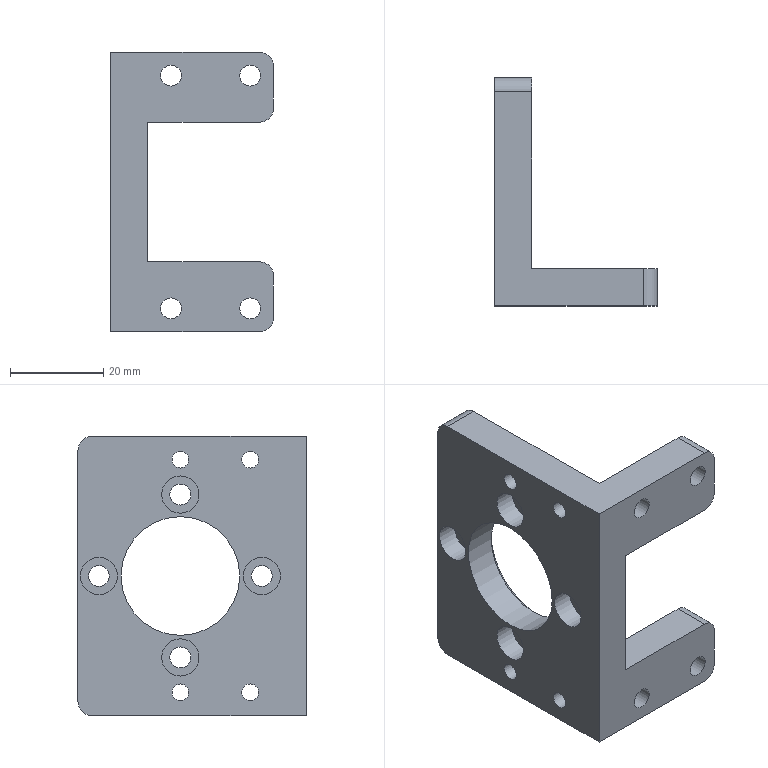CAM job | NX | 3+2 milling, drilling | part box 35 x 49 x 60 mm | stock box 40 x 50 x 65 mm
Tools:
number,name,description,diameter,corner_radius,flute_length,length,flutes
4,D4,平底铣刀-粗,4.0,0.0,25.0,75.0,2
9,D10,平底铣刀-粗,10.0,0.0,35.0,75.0,2
10,D10-J,平底铣刀-精,10.0,0.0,35.0,75.0,2
1,D80R0.8飞刀,圆鼻刀-粗,80.0,0.8,50.0,75.0,2
17,D6R0.5-J,圆鼻刀-精,6.0,0.5,50.0,75.0,2
1,D80R0.8飞刀-J,圆鼻刀-精,80.0,0.8,50.0,75.0,2
2,D6倒角刀,倒角刀,6.0,0.0,3.0,25.0,2
17,ZT3.6,钻头,3.6,0.0,35.0,50.0,2
11,ZT4.5,钻头,4.5,0.0,35.0,50.0,2
18,ZT10,钻头,10.0,0.0,35.0,50.0,2
Operations:
program,operation,operation_type,tool,method,geometry_group,spindle_rpm,surface_speed,feed_per_tooth,feed_cut,feed_plunge,cut_length_mm,path_length_mm,cut_time_min,machine_time_min
B,底壁铣飞面一刀开粗_COPY,VolumeBased25DMillingOperation,D80R0.8飞刀,分层开粗-切深K-步距G,W-B,2800.0,703.696,0.5357,3000.0,100.0,1513.746,3025.967,0.5046,0.6558
B,底壁铣飞面一刀精光_COPY,VolumeBased25DMillingOperation,D80R0.8飞刀-J,侧刃精光-切深K-步距G,W-B,4000.0,1005.28,0.125,1000.0,100.0,167.998,203.998,0.168,0.1716
B,底壁铣分层开粗-中_COPY,VolumeBased25DMillingOperation,D10,分层开粗-切深K-步距G,W-B,8000.0,251.327,0.3125,5000.0,100.0,28044.512,28961.091,5.609,5.701
B,等高精光往复爬面_COPY_COPY,ZLevelMilling,D10,等高爬面-切深K-步距G,W-B,7000.0,131.947,0.3214,4500.0,100.0,1154.433,1400.109,0.2565,0.2811
B,铣沉头_1,CylinderMilling,D4,METHOD,W-B,8000.0,100.531,0.075,1200.0,100.0,467.722,936.122,0.3898,0.4366
B,铣孔_1,CylinderMilling,D4,METHOD,W-B,8000.0,100.531,0.0375,600.0,100.0,37.039,520.239,0.0617,0.1101
B,等高精光往复爬面_COPY,ZLevelMilling,D6R0.5-J,等高爬面-切深K-步距G,W-B,7000.0,131.947,0.3214,4500.0,100.0,2411.018,2616.21,0.5358,0.5563
B,钻倒角_2,Operation,D6倒角刀,METHOD,W-B,8000.0,150.796,0.0625,1000.0,0.0,22.2,222.19,0.0222,0.0422
B,平面去毛刺6X45L_COPY,SurfaceContour,D6倒角刀,爬面_倒角-切深0-步距G,W-B,6500.0,122.519,0.1154,1500.0,100.0,514.645,1211.426,0.3431,0.4128
B,底壁铣倒角_COPY,VolumeBased25DMillingOperation,D6倒角刀,爬面_倒角-切深0-步距G,W-B,6500.0,122.519,0.1154,1500.0,100.0,323.434,417.834,0.2156,0.2251
B,底壁铣精光底面-中_COPY,VolumeBased25DMillingOperation,D10-J,精光步距切深关,W-B,7000.0,175.0,0.0536,1500.0,100.0,621.716,701.716,0.4145,0.4225
B,底壁铣精光侧面-中-选底面_COPY,VolumeBased25DMillingOperation,D10-J,侧刃精光-切深K-步距G,W-B,8000.0,251.32,0.0625,1000.0,100.0,206.727,603.008,0.2067,0.2464
A,顶面开粗,FaceMilling,D80R0.8飞刀,分层开粗-切深K-步距G,W-A,4000.0,1005.31,0.375,3000.0,100.0,154.0,189.8,0.0513,0.0549
A,顶面,FaceMilling,D80R0.8飞刀,侧刃精光-切深K-步距G,W-A,4000.0,1005.31,0.125,1000.0,100.0,154.0,190.0,0.154,0.1576
A,外形粗_2,VolumeBased25DMillingOperation,D10,METHOD,W-A,8000.0,251.327,0.3125,5000.0,80.0,11385.133,11458.933,2.277,2.284
A,底壁铣螺旋开粗-中_COPY,VolumeBased25DMillingOperation,D10,分层开粗-切深K-步距G,W-A,8000.0,251.32,0.25,4000.0,100.0,789.619,836.119,0.1974,0.2021
A,打点0.8,Operation,D6倒角刀,METHOD,W-A,8000.0,150.796,0.0312,500.0,0.0,1.8,43.6,0.0036,0.0078
A,打点-深0.8,Operation,D6倒角刀,NONE,W-A,8000.0,150.796,0.0312,500.0,90.0,14.4,195.682,0.0288,0.0469
A,通孔-3-4,Operation,ZT3.6,NONE,W-A,3000.0,33.929,0.02,120.0,90.0,52.0,227.077,0.4333,0.4508
A,沉头孔-钻孔0段,Operation,ZT4.5,NONE,W-A,2800.0,39.584,0.0179,100.0,90.0,49.408,216.122,0.4941,0.5107
A,通孔-10-12.5,Operation,ZT10,NONE,W-A,1500.0,120.166,0.05,150.0,90.0,14.004,68.009,0.0934,0.0988
A,铣孔开粗D4_1,CylinderMilling,D4,NONE,W-A,8000.0,100.531,0.075,1200.0,100.0,883.672,1134.318,0.7364,0.7615
A,铣孔精光D4_1,CylinderMilling,D4,精光步距切深关,W-A,8000.0,100.531,0.0312,500.0,100.0,130.348,380.995,0.2607,0.2858
A,仅选体,SurfaceContour,D6倒角刀,METHOD,W-A,8000.0,150.796,0.1875,3000.0,100.0,313.876,416.62,0.1046,0.1149
A,钻倒角_1,Operation,D6倒角刀,METHOD,W-A,8000.0,150.796,0.0312,500.0,0.0,20.4,170.484,0.0408,0.0558
A,铣倒角_1,PlanarMilling,D6倒角刀,NONE,W-A,8000.0,150.796,0.0312,500.0,100.0,135.871,361.016,0.2717,0.2943
A,铣倒角_2,PlanarMilling,D6倒角刀,METHOD,W-A,8000.0,150.796,0.05,800.0,100.0,86.137,127.137,0.1077,0.1118
A,底壁铣精光侧面-中_COPY,VolumeBased25DMillingOperation,D10-J,侧刃精光-切深K-步距G,W-A,8000.0,251.32,0.0625,1000.0,100.0,57.572,92.172,0.0576,0.061
A,外形半精_2,VolumeBased25DMillingOperation,D10-J,METHOD,W-A,8000.0,251.327,0.0625,1000.0,100.0,755.397,1018.626,0.7554,0.7817